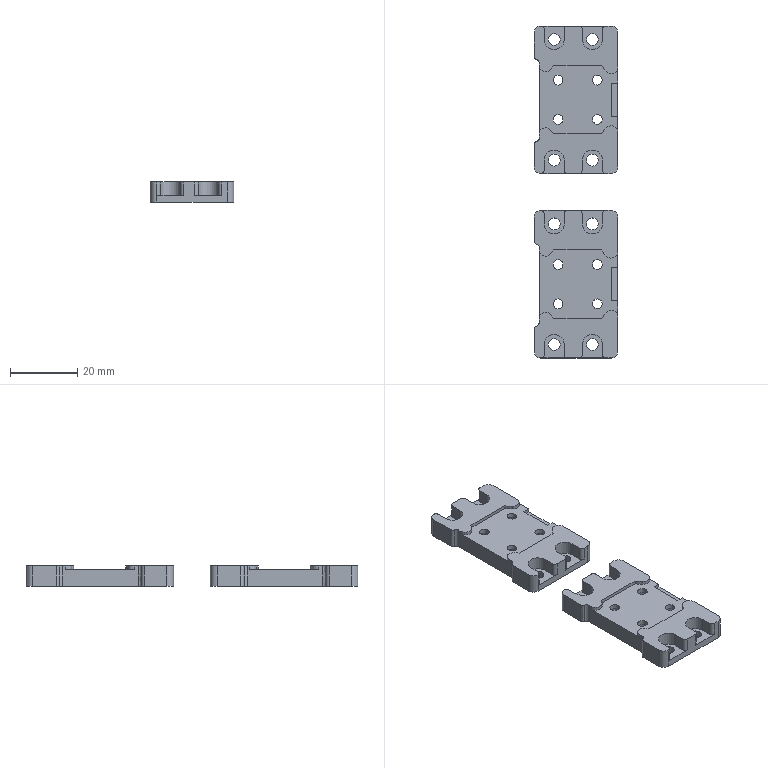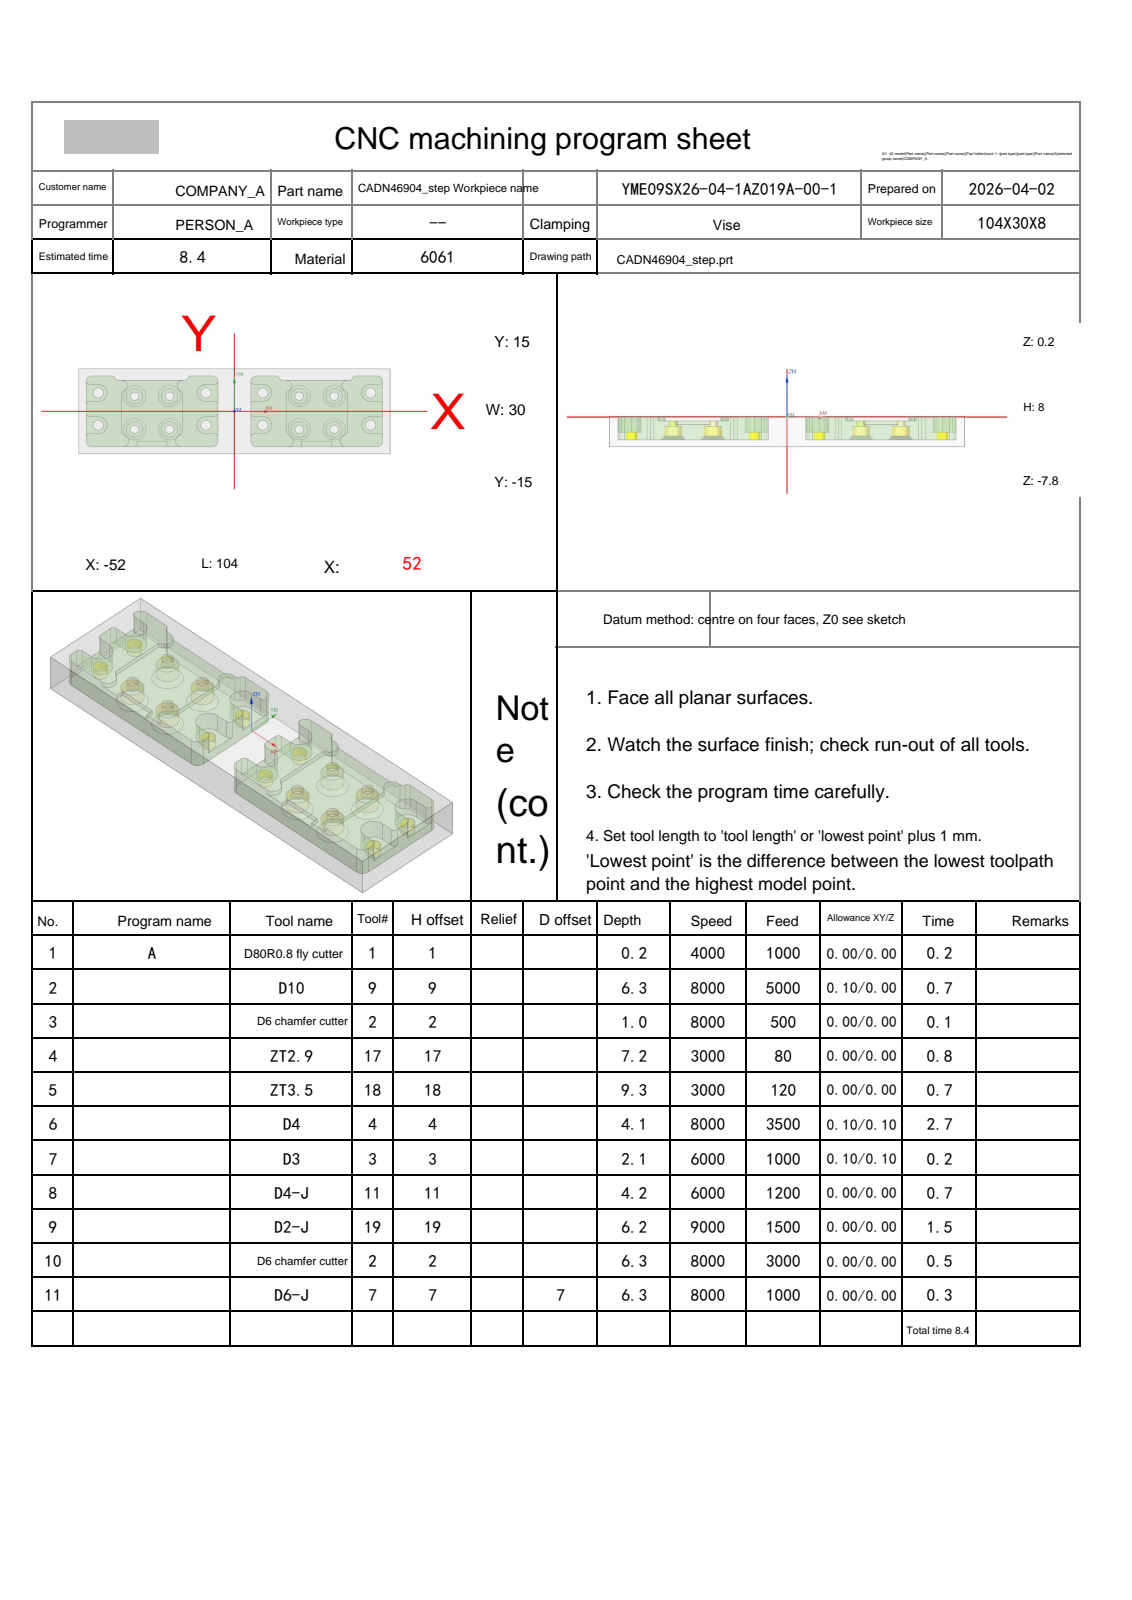NC program | NX | posted by the shop | part box 25 x 99 x 6 mm
Lines 2901 to 3253 of 9316:
N8 T11 M06
(D4-J  D=4. R=0. H=11 ce=0.30 di=0.00)
G00 G90 G54 X-27.5 Y-15.5 M03 S6000
G43 H11 Z20.
M08
Z-.5
G01 Z-1. F1200.
Y-10.9
X-32.1
Y-12.9
X-33.73
G03 X-32.998 Y-10.5 I-3.568 J2.4
X-34.286 Y-7.431 I-4.3 J0.0
X-35.4 Y-6.446 I-10.016 J-10.206
G01 Y5.446
G03 X-35.071 Y5.716 I-8.902 J11.191
X-33.547 Y9. I-2.776 J3.284
X-34.279 Y11.4 I-4.3 J0.0
G01 X-20.721
G03 X-21.453 Y9. I3.568 J-2.4
X-19.929 Y5.716 I4.3 J0.0
X-19.6 Y5.446 I9.231 J10.921
G01 Y-6.446
G03 X-20.714 Y-7.431 I8.902 J-11.191
X-22.002 Y-10.5 I3.012 J-3.069
X-21.27 Y-12.9 I4.3 J0.0
G01 X-22.9
Y-10.9
X-27.5
Y-8.1
X-30.616
G03 X-32.325 Y-5.433 I-6.682 J-2.4
X-32.6 Y-5.169 I-11.977 J-12.205
G01 Y4.217
G03 X-30.758 Y8.6 I-5.247 J4.783
G01 X-24.242
G03 X-22.4 Y4.217 I7.089 J.4
G01 Y-5.169
G03 X-22.675 Y-5.433 I11.702 J-12.469
X-24.384 Y-8.1 I4.973 J-5.067
G01 X-27.5
Y-5.3
X-28.874
G03 X-29.8 Y-4.035 I-8.424 J-5.2
G01 Y3.233
G03 X-28.478 Y5.8 I-8.047 J5.767
G01 X-26.522
G03 X-25.2 Y3.233 I9.369 J3.2
G01 Y-4.035
G03 X-26.126 Y-5.3 I7.498 J-6.465
G01 X-27.5
Y-3.5
X-27.923
X-28. Y-3.398
Y2.681
G03 X-27.5 Y3.538 I-9.847 J6.319
X-27. Y2.681 I10.347 J5.462
G01 Y-3.398
X-27.077 Y-3.5
X-27.5
X-27.923
X-27.969 Y-3.438
X-29.883 Y-4.887
Z-.5
G00 Z20.
X27.5 Y-15.5
Z-.5
G01 Z-1.
Y-10.9
X22.9
Y-12.9
X21.27
G03 X22.002 Y-10.5 I-3.568 J2.4
X20.714 Y-7.431 I-4.3 J0.0
X19.6 Y-6.446 I-10.016 J-10.206
G01 Y5.446
G03 X19.929 Y5.716 I-8.902 J11.191
X21.453 Y9. I-2.776 J3.284
X20.721 Y11.4 I-4.3 J0.0
G01 X34.279
G03 X33.547 Y9. I3.568 J-2.4
X35.071 Y5.716 I4.3 J0.0
X35.4 Y5.446 I9.231 J10.921
G01 Y-6.446
G03 X34.286 Y-7.431 I8.902 J-11.191
X32.998 Y-10.5 I3.012 J-3.069
X33.73 Y-12.9 I4.3 J0.0
G01 X32.1
Y-10.9
X27.5
Y-8.1
X24.384
G03 X22.675 Y-5.433 I-6.682 J-2.4
X22.4 Y-5.169 I-11.977 J-12.205
G01 Y4.217
G03 X24.242 Y8.6 I-5.247 J4.783
G01 X30.758
G03 X32.6 Y4.217 I7.089 J.4
G01 Y-5.169
G03 X32.325 Y-5.433 I11.702 J-12.469
X30.616 Y-8.1 I4.973 J-5.067
G01 X27.5
Y-5.3
X26.126
G03 X25.2 Y-4.035 I-8.424 J-5.2
G01 Y3.233
G03 X26.522 Y5.8 I-8.047 J5.767
G01 X28.478
G03 X29.8 Y3.233 I9.369 J3.2
G01 Y-4.035
G03 X28.874 Y-5.3 I7.498 J-6.465
G01 X27.5
Y-3.5
X27.077
X27. Y-3.398
Y2.681
G03 X27.5 Y3.538 I-9.847 J6.319
X28. Y2.681 I10.347 J5.462
G01 Y-3.398
X27.923 Y-3.5
X27.5
X27.077
X27.031 Y-3.438
X25.117 Y-4.887
Z-.5
G00 Z20.
G00 G90 X-14.902 Y-15.6 M03 S6000
Z20.
Z-.495
G01 Z-.995 F1200.
G41 D11
Y-15.5
G03 X-15.902 Y-14.5 I-1. J0.0
G01 X-17.702
G02 X-21.702 Y-10.5 I0.0 J4.
X-20.504 Y-7.645 I4. J0.0
X-19.3 Y-6.592 I9.806 J-9.992
G01 Y5.592
G02 X-19.735 Y5.945 I8.602 J11.045
X-21.153 Y9. I2.582 J3.055
X-17.162 Y13. I4. J0.0
X-16.49 Y13.8 I2.598 J-1.5
G03 X-16.132 Y14.567 I-.642 J.767
X-16.291 Y15.108 I-1. J0.0
G01 G40 X-16.345 Y15.192
Z-.495
G00 Z20.
X-39.155
Z-.495
G01 Z-.995
G41 D11
X-39.209 Y15.108
G03 X-39.368 Y14.567 I.841 J-.541
X-39.01 Y13.8 I1. J0.0
G02 X-38.338 Y13. I-1.926 J-2.3
G01 X-37.847
G02 X-33.847 Y9. I0.0 J-4.
X-35.265 Y5.945 I-4. J0.0
X-35.7 Y5.592 I-9.038 J10.692
G01 Y-6.592
G02 X-34.496 Y-7.645 I-8.602 J-11.045
X-33.298 Y-10.5 I-2.802 J-2.855
X-37.298 Y-14.5 I-4. J0.0
G01 X-39.098
G03 X-40.098 Y-15.5 I0.0 J-1.
G01 G40 Y-15.6
Z-.495
G00 Z20.
X15.845 Y15.192
Z-.495
G01 Z-.995
G41 D11
X15.791 Y15.108
G03 X15.632 Y14.567 I.841 J-.541
X15.99 Y13.8 I1. J0.0
G02 X16.662 Y13. I-1.926 J-2.3
G01 X17.153
G02 X21.153 Y9. I0.0 J-4.
X19.735 Y5.945 I-4. J0.0
X19.3 Y5.592 I-9.038 J10.692
G01 Y-6.592
G02 X20.504 Y-7.645 I-8.602 J-11.045
X21.702 Y-10.5 I-2.802 J-2.855
X17.702 Y-14.5 I-4. J0.0
G01 X15.902
G03 X14.902 Y-15.5 I0.0 J-1.
G01 G40 Y-15.6
Z-.495
G00 Z20.
X40.098
Z-.495
G01 Z-.995
G41 D11
Y-15.5
G03 X39.098 Y-14.5 I-1. J0.0
G01 X37.298
G02 X33.298 Y-10.5 I0.0 J4.
X34.496 Y-7.645 I4. J0.0
X35.7 Y-6.592 I9.806 J-9.992
G01 Y5.592
G02 X35.265 Y5.945 I8.602 J11.045
X33.847 Y9. I2.582 J3.055
X37.838 Y13. I4. J0.0
X38.51 Y13.8 I2.598 J-1.5
G03 X38.868 Y14.567 I-.642 J.767
X38.709 Y15.108 I-1. J0.0
G01 G40 X38.655 Y15.192
Z-.495
G00 Z20.
G00 G90 X51.512 Y13.647 M03 S6000
Z20.
Z-3.5
G01 Z-4. F1200.
G41 D11
X51.428 Y13.594
G03 X50.965 Y12.75 I.537 J-.844
X51.072 Y12.3 I1. J0.0
G02 X51.5 Y10.5 I-3.572 J-1.8
X48.5 Y7.5 I-3. J0.0
G01 X45.5
G03 X44.5 Y6.5 I0.0 J-1.
X45.5 Y5.5 I1. J0.0
G01 X48.5
G02 X51.5 Y2.5 I0.0 J-3.
G01 Y-.881
G02 X48.5 Y-3.881 I-3. J0.0
G01 X45.5
G03 X44.5 Y-4.881 I0.0 J-1.
X45.5 Y-5.881 I1. J0.0
G01 X48.5
G02 X51.5 Y-8.881 I0.0 J-3.
G01 Y-10.5
X51.496 Y-10.681
X51.495 Y-10.726
G03 X52.35 Y-11.715 I1. J0.0
G01 G40 X52.449 Y-11.73
Z-3.5
G00 Z20.
X2.551
Z-3.5
G01 Z-4.
G41 D11
X2.65 Y-11.715
G03 X3.505 Y-10.726 I-.145 J.989
G01 X3.504 Y-10.681
X3.5 Y-10.5
Y-8.881
G02 X6.5 Y-5.881 I3. J0.0
G01 X9.5
G03 X10.5 Y-4.881 I0.0 J1.
X9.5 Y-3.881 I-1. J0.0
G01 X6.5
G02 X3.5 Y-.881 I0.0 J3.
G01 Y2.5
G02 X6.5 Y5.5 I3. J0.0
G01 X9.5
G03 X10.5 Y6.5 I0.0 J1.
X9.5 Y7.5 I-1. J0.0
G01 X6.5
G02 X3.5 Y10.5 I0.0 J3.
X3.517 Y10.864 I4. J0.0
G01 X3.521 Y10.955
G03 X2.711 Y11.937 I-1. J0.0
G01 G40 X2.613 Y11.956
Z-3.5
G00 Z20.
X2.402 Y10.631
Z-3.5
G01 Z-4.
G41 D11
X2.501 Y10.619
X2.625 Y10.611
G03 X3.6 Y11.389 I0.0 J1.
G02 X3.928 Y12.3 I3.9 J-.889
G03 X4.035 Y12.75 I-.893 J.45
X3.572 Y13.594 I-1. J0.0
G01 G40 X3.488 Y13.647
Z-3.5
G00 Z20.
X-3.488
Z-3.5
G01 Z-4.
G41 D11
X-3.572 Y13.594
G03 X-4.035 Y12.75 I.537 J-.844
X-3.928 Y12.3 I1. J0.0
G02 X-3.5 Y10.5 I-3.572 J-1.8
X-6.5 Y7.5 I-3. J0.0
G01 X-9.5
G03 X-10.5 Y6.5 I0.0 J-1.
X-9.5 Y5.5 I1. J0.0
G01 X-6.5
G02 X-3.5 Y2.5 I0.0 J-3.
G01 Y-.881
G02 X-6.5 Y-3.881 I-3. J0.0
G01 X-9.5
G03 X-10.5 Y-4.881 I0.0 J-1.
X-9.5 Y-5.881 I1. J0.0
G01 X-6.5
G02 X-3.5 Y-8.881 I0.0 J-3.
G01 Y-10.5
X-3.504 Y-10.681
X-3.505 Y-10.726
G03 X-2.65 Y-11.715 I1. J0.0
G01 G40 X-2.551 Y-11.73
Z-3.5
G00 Z20.
X-52.449
Z-3.5
G01 Z-4.
G41 D11
X-52.35 Y-11.715
G03 X-51.495 Y-10.726 I-.145 J.989
G01 X-51.496 Y-10.681
X-51.5 Y-10.5
Y-8.881
G02 X-48.5 Y-5.881 I3. J0.0
G01 X-45.5
G03 X-44.5 Y-4.881 I0.0 J1.
X-45.5 Y-3.881 I-1. J0.0
G01 X-48.5
G02 X-51.5 Y-.881 I0.0 J3.
G01 Y2.5
G02 X-48.5 Y5.5 I3. J0.0
G01 X-45.5
G03 X-44.5 Y6.5 I0.0 J1.
X-45.5 Y7.5 I-1. J0.0
G01 X-48.5
G02 X-51.5 Y10.5 I0.0 J3.
X-51.484 Y10.858 I4. J0.0
G01 X-51.48 Y10.948
G03 X-52.291 Y11.93 I-1. J0.0
G01 G40 X-52.389 Y11.949
Z-3.5
G00 Z20.
X-52.598 Y10.631
Z-3.5
G01 Z-4.
G41 D11
X-52.499 Y10.619
X-52.375 Y10.611
G03 X-51.4 Y11.389 I0.0 J1.
G02 X-51.072 Y12.3 I3.9 J-.889
G03 X-50.965 Y12.75 I-.893 J.45
X-51.428 Y13.594 I-1. J0.0
G01 G40 X-51.512 Y13.647
Z-3.5
G00 Z20.
G91 G28 Z0.0
M05
M09
G91 G28 Z0.0
M01